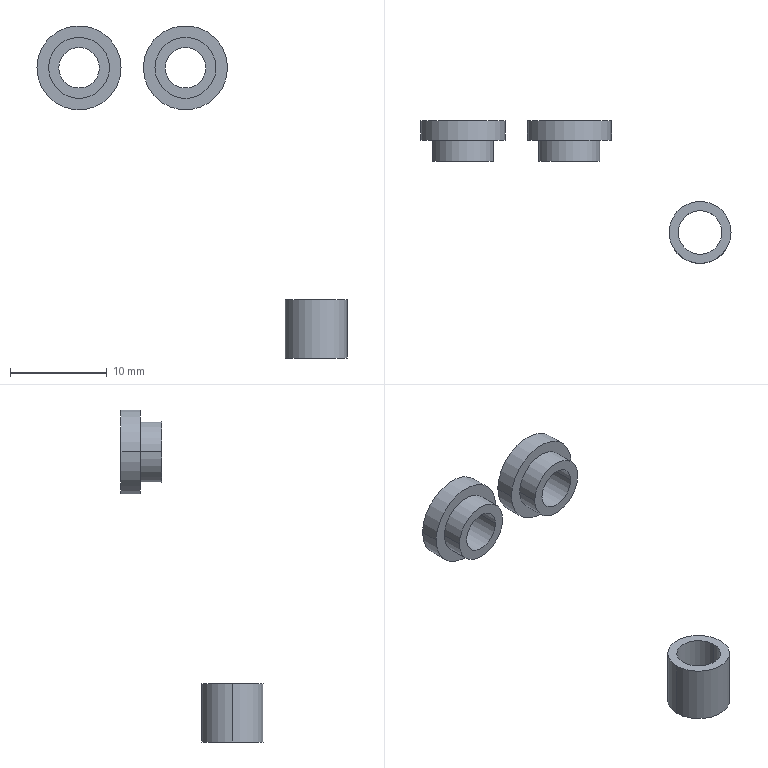Part | NX | features BREP 3 | 3 solids | 24 faces | box 32.05 x 14.7 x 34.343 mm | volume 356.162 mm3 | cylinder 16 | plane 8 | commonest cylinder face diameters 4.2 x4 6.3 x4 8.7 x4 4.5 x2 6.4 x2
STEP:
#1=CARTESIAN_POINT('',(49.941,-46.741,33.83));
#2=VERTEX_POINT('',#1);
#3=CARTESIAN_POINT('',(43.541,-46.741,33.83));
#4=VERTEX_POINT('',#3);
#5=CARTESIAN_POINT('',(46.741,-46.741,33.83));
#6=DIRECTION('',(0.,0.,1.));
#7=DIRECTION('',(1.,0.,0.));
#8=AXIS2_PLACEMENT_3D('',#5,#6,#7);
#9=CIRCLE('',#8,3.2);
#10=EDGE_CURVE('',#2,#4,#9,.T.);
#11=ORIENTED_EDGE('',*,*,#10,.T.);
#12=CARTESIAN_POINT('',(46.741,-46.741,33.83));
#13=DIRECTION('',(0.,0.,1.));
#14=DIRECTION('',(-1.,0.,0.));
#15=AXIS2_PLACEMENT_3D('',#12,#13,#14);
#16=CIRCLE('',#15,3.2);
#17=EDGE_CURVE('',#4,#2,#16,.T.);
#18=ORIENTED_EDGE('',*,*,#17,.T.);
#19=EDGE_LOOP('',(#11,#18));
#20=FACE_BOUND('',#19,.T.);
#21=CARTESIAN_POINT('',(48.991,-46.741,33.83));
#22=VERTEX_POINT('',#21);
#23=CARTESIAN_POINT('',(44.491,-46.741,33.83));
#24=VERTEX_POINT('',#23);
#25=CARTESIAN_POINT('',(46.741,-46.741,33.83));
#26=DIRECTION('',(0.,0.,-1.));
#27=DIRECTION('',(1.,0.,0.));
#28=AXIS2_PLACEMENT_3D('',#25,#26,#27);
#29=CIRCLE('',#28,2.25);
#30=EDGE_CURVE('',#22,#24,#29,.T.);
#31=ORIENTED_EDGE('',*,*,#30,.T.);
#32=CARTESIAN_POINT('',(46.741,-46.741,33.83));
#33=DIRECTION('',(0.,0.,-1.));
#34=DIRECTION('',(-1.,0.,0.));
#35=AXIS2_PLACEMENT_3D('',#32,#33,#34);
#36=CIRCLE('',#35,2.25);
#37=EDGE_CURVE('',#24,#22,#36,.T.);
#38=ORIENTED_EDGE('',*,*,#37,.T.);
#39=EDGE_LOOP('',(#31,#38));
#40=FACE_BOUND('',#39,.T.);
#41=CARTESIAN_POINT('',(0.,0.,33.83));
#42=DIRECTION('',(0.,0.,1.));
#43=DIRECTION('',(1.,0.,0.));
#44=AXIS2_PLACEMENT_3D('',#41,#42,#43);
#45=PLANE('',#44);
#46=ADVANCED_FACE('',(#20,#40),#45,.T.);
#47=CARTESIAN_POINT('',(49.941,-46.741,27.83));
#48=VERTEX_POINT('',#47);
#49=CARTESIAN_POINT('',(43.541,-46.741,27.83));
#50=VERTEX_POINT('',#49);
#51=CARTESIAN_POINT('',(46.741,-46.741,27.83));
#52=DIRECTION('',(0.,0.,-1.));
#53=DIRECTION('',(1.,0.,0.));
#54=AXIS2_PLACEMENT_3D('',#51,#52,#53);
#55=CIRCLE('',#54,3.2);
#56=EDGE_CURVE('',#48,#50,#55,.T.);
#57=ORIENTED_EDGE('',*,*,#56,.F.);
#58=CARTESIAN_POINT('',(49.941,-46.741,33.83));
#59=DIRECTION('',(0.,0.,-1.));
#60=VECTOR('',#59,1000.);
#61=LINE('',#58,#60);
#62=EDGE_CURVE('',#2,#48,#61,.T.);
#63=ORIENTED_EDGE('',*,*,#62,.F.);
#64=ORIENTED_EDGE('',*,*,#17,.F.);
#65=CARTESIAN_POINT('',(43.541,-46.741,33.83));
#66=DIRECTION('',(0.,0.,-1.));
#67=VECTOR('',#66,1000.);
#68=LINE('',#65,#67);
#69=EDGE_CURVE('',#4,#50,#68,.T.);
#70=ORIENTED_EDGE('',*,*,#69,.T.);
#71=EDGE_LOOP('',(#57,#63,#64,#70));
#72=FACE_BOUND('',#71,.T.);
#73=CARTESIAN_POINT('',(46.741,-46.741,33.83));
#74=DIRECTION('',(0.,0.,1.));
#75=DIRECTION('',(1.,0.,0.));
#76=AXIS2_PLACEMENT_3D('',#73,#74,#75);
#77=CYLINDRICAL_SURFACE('',#76,3.2);
#78=ADVANCED_FACE('',(#72),#77,.T.);
#79=CARTESIAN_POINT('',(46.741,-46.741,27.83));
#80=DIRECTION('',(0.,0.,-1.));
#81=DIRECTION('',(-1.,0.,0.));
#82=AXIS2_PLACEMENT_3D('',#79,#80,#81);
#83=CIRCLE('',#82,3.2);
#84=EDGE_CURVE('',#50,#48,#83,.T.);
#85=ORIENTED_EDGE('',*,*,#84,.F.);
#86=ORIENTED_EDGE('',*,*,#69,.F.);
#87=ORIENTED_EDGE('',*,*,#10,.F.);
#88=ORIENTED_EDGE('',*,*,#62,.T.);
#89=EDGE_LOOP('',(#85,#86,#87,#88));
#90=FACE_BOUND('',#89,.T.);
#91=CARTESIAN_POINT('',(46.741,-46.741,33.83));
#92=DIRECTION('',(0.,0.,1.));
#93=DIRECTION('',(1.,0.,0.));
#94=AXIS2_PLACEMENT_3D('',#91,#92,#93);
#95=CYLINDRICAL_SURFACE('',#94,3.2);
#96=ADVANCED_FACE('',(#90),#95,.T.);
#97=ORIENTED_EDGE('',*,*,#84,.T.);
#98=ORIENTED_EDGE('',*,*,#56,.T.);
#99=EDGE_LOOP('',(#97,#98));
#100=FACE_BOUND('',#99,.T.);
#101=CARTESIAN_POINT('',(44.491,-46.741,27.83));
#102=VERTEX_POINT('',#101);
#103=CARTESIAN_POINT('',(48.991,-46.741,27.83));
#104=VERTEX_POINT('',#103);
#105=CARTESIAN_POINT('',(46.741,-46.741,27.83));
#106=DIRECTION('',(0.,0.,1.));
#107=DIRECTION('',(-1.,0.,0.));
#108=AXIS2_PLACEMENT_3D('',#105,#106,#107);
#109=CIRCLE('',#108,2.25);
#110=EDGE_CURVE('',#102,#104,#109,.T.);
#111=ORIENTED_EDGE('',*,*,#110,.T.);
#112=CARTESIAN_POINT('',(46.741,-46.741,27.83));
#113=DIRECTION('',(0.,0.,1.));
#114=DIRECTION('',(1.,0.,0.));
#115=AXIS2_PLACEMENT_3D('',#112,#113,#114);
#116=CIRCLE('',#115,2.25);
#117=EDGE_CURVE('',#104,#102,#116,.T.);
#118=ORIENTED_EDGE('',*,*,#117,.T.);
#119=EDGE_LOOP('',(#111,#118));
#120=FACE_BOUND('',#119,.T.);
#121=CARTESIAN_POINT('',(0.,0.,27.83));
#122=DIRECTION('',(0.,0.,1.));
#123=DIRECTION('',(1.,0.,0.));
#124=AXIS2_PLACEMENT_3D('',#121,#122,#123);
#125=PLANE('',#124);
#126=ADVANCED_FACE('',(#100,#120),#125,.F.);
#127=ORIENTED_EDGE('',*,*,#117,.F.);
#128=CARTESIAN_POINT('',(48.991,-46.741,33.83));
#129=DIRECTION('',(0.,0.,-1.));
#130=VECTOR('',#129,1000.);
#131=LINE('',#128,#130);
#132=EDGE_CURVE('',#22,#104,#131,.T.);
#133=ORIENTED_EDGE('',*,*,#132,.F.);
#134=ORIENTED_EDGE('',*,*,#37,.F.);
#135=CARTESIAN_POINT('',(44.491,-46.741,33.83));
#136=DIRECTION('',(0.,0.,-1.));
#137=VECTOR('',#136,1000.);
#138=LINE('',#135,#137);
#139=EDGE_CURVE('',#24,#102,#138,.T.);
#140=ORIENTED_EDGE('',*,*,#139,.T.);
#141=EDGE_LOOP('',(#127,#133,#134,#140));
#142=FACE_BOUND('',#141,.T.);
#143=CARTESIAN_POINT('',(46.741,-46.741,33.83));
#144=DIRECTION('',(0.,0.,1.));
#145=DIRECTION('',(1.,0.,0.));
#146=AXIS2_PLACEMENT_3D('',#143,#144,#145);
#147=CYLINDRICAL_SURFACE('',#146,2.25);
#148=ADVANCED_FACE('',(#142),#147,.F.);
#149=ORIENTED_EDGE('',*,*,#110,.F.);
#150=ORIENTED_EDGE('',*,*,#139,.F.);
#151=ORIENTED_EDGE('',*,*,#30,.F.);
#152=ORIENTED_EDGE('',*,*,#132,.T.);
#153=EDGE_LOOP('',(#149,#150,#151,#152));
#154=FACE_BOUND('',#153,.T.);
#155=CARTESIAN_POINT('',(46.741,-46.741,33.83));
#156=DIRECTION('',(0.,0.,1.));
#157=DIRECTION('',(1.,0.,0.));
#158=AXIS2_PLACEMENT_3D('',#155,#156,#157);
#159=CYLINDRICAL_SURFACE('',#158,2.25);
#160=ADVANCED_FACE('',(#154),#159,.F.);
#161=CLOSED_SHELL('',(#46,#78,#96,#126,#148,#160));
#162=MANIFOLD_SOLID_BREP('',#161);
#163=CARTESIAN_POINT('',(26.591,-37.241,57.823));
#164=VERTEX_POINT('',#163);
#165=CARTESIAN_POINT('',(17.891,-37.241,57.823));
#166=VERTEX_POINT('',#165);
#167=CARTESIAN_POINT('',(22.241,-37.241,57.823));
#168=DIRECTION('',(0.,1.,0.));
#169=DIRECTION('',(1.,0.,0.));
#170=AXIS2_PLACEMENT_3D('',#167,#168,#169);
#171=CIRCLE('',#170,4.35);
#172=EDGE_CURVE('',#164,#166,#171,.T.);
#173=ORIENTED_EDGE('',*,*,#172,.F.);
#174=CARTESIAN_POINT('',(22.241,-37.241,57.823));
#175=DIRECTION('',(0.,1.,0.));
#176=DIRECTION('',(-1.,0.,0.));
#177=AXIS2_PLACEMENT_3D('',#174,#175,#176);
#178=CIRCLE('',#177,4.35);
#179=EDGE_CURVE('',#166,#164,#178,.T.);
#180=ORIENTED_EDGE('',*,*,#179,.F.);
#181=EDGE_LOOP('',(#173,#180));
#182=FACE_BOUND('',#181,.T.);
#183=CARTESIAN_POINT('',(19.091,-37.241,57.823));
#184=VERTEX_POINT('',#183);
#185=CARTESIAN_POINT('',(25.391,-37.241,57.823));
#186=VERTEX_POINT('',#185);
#187=CARTESIAN_POINT('',(22.241,-37.241,57.823));
#188=DIRECTION('',(0.,-1.,0.));
#189=DIRECTION('',(-1.,0.,0.));
#190=AXIS2_PLACEMENT_3D('',#187,#188,#189);
#191=CIRCLE('',#190,3.15);
#192=EDGE_CURVE('',#184,#186,#191,.T.);
#193=ORIENTED_EDGE('',*,*,#192,.F.);
#194=CARTESIAN_POINT('',(22.241,-37.241,57.823));
#195=DIRECTION('',(0.,-1.,0.));
#196=DIRECTION('',(1.,0.,0.));
#197=AXIS2_PLACEMENT_3D('',#194,#195,#196);
#198=CIRCLE('',#197,3.15);
#199=EDGE_CURVE('',#186,#184,#198,.T.);
#200=ORIENTED_EDGE('',*,*,#199,.F.);
#201=EDGE_LOOP('',(#193,#200));
#202=FACE_BOUND('',#201,.T.);
#203=CARTESIAN_POINT('',(0.,-37.241,0.));
#204=DIRECTION('',(0.,1.,0.));
#205=DIRECTION('',(1.,0.,0.));
#206=AXIS2_PLACEMENT_3D('',#203,#204,#205);
#207=PLANE('',#206);
#208=ADVANCED_FACE('',(#182,#202),#207,.F.);
#209=CARTESIAN_POINT('',(26.591,-35.241,57.823));
#210=VERTEX_POINT('',#209);
#211=CARTESIAN_POINT('',(26.591,-37.241,57.823));
#212=DIRECTION('',(0.,-1.,0.));
#213=VECTOR('',#212,1000.);
#214=LINE('',#211,#213);
#215=EDGE_CURVE('',#210,#164,#214,.T.);
#216=ORIENTED_EDGE('',*,*,#215,.F.);
#217=CARTESIAN_POINT('',(17.891,-35.241,57.823));
#218=VERTEX_POINT('',#217);
#219=CARTESIAN_POINT('',(22.241,-35.241,57.823));
#220=DIRECTION('',(0.,1.,0.));
#221=DIRECTION('',(-1.,0.,0.));
#222=AXIS2_PLACEMENT_3D('',#219,#220,#221);
#223=CIRCLE('',#222,4.35);
#224=EDGE_CURVE('',#218,#210,#223,.T.);
#225=ORIENTED_EDGE('',*,*,#224,.F.);
#226=CARTESIAN_POINT('',(17.891,-37.241,57.823));
#227=DIRECTION('',(0.,-1.,0.));
#228=VECTOR('',#227,1000.);
#229=LINE('',#226,#228);
#230=EDGE_CURVE('',#218,#166,#229,.T.);
#231=ORIENTED_EDGE('',*,*,#230,.T.);
#232=ORIENTED_EDGE('',*,*,#179,.T.);
#233=EDGE_LOOP('',(#216,#225,#231,#232));
#234=FACE_BOUND('',#233,.T.);
#235=CARTESIAN_POINT('',(22.241,-37.241,57.823));
#236=DIRECTION('',(0.,1.,0.));
#237=DIRECTION('',(1.,0.,0.));
#238=AXIS2_PLACEMENT_3D('',#235,#236,#237);
#239=CYLINDRICAL_SURFACE('',#238,4.35);
#240=ADVANCED_FACE('',(#234),#239,.T.);
#241=ORIENTED_EDGE('',*,*,#230,.F.);
#242=CARTESIAN_POINT('',(22.241,-35.241,57.823));
#243=DIRECTION('',(0.,1.,0.));
#244=DIRECTION('',(1.,0.,0.));
#245=AXIS2_PLACEMENT_3D('',#242,#243,#244);
#246=CIRCLE('',#245,4.35);
#247=EDGE_CURVE('',#210,#218,#246,.T.);
#248=ORIENTED_EDGE('',*,*,#247,.F.);
#249=ORIENTED_EDGE('',*,*,#215,.T.);
#250=ORIENTED_EDGE('',*,*,#172,.T.);
#251=EDGE_LOOP('',(#241,#248,#249,#250));
#252=FACE_BOUND('',#251,.T.);
#253=CARTESIAN_POINT('',(22.241,-37.241,57.823));
#254=DIRECTION('',(0.,1.,0.));
#255=DIRECTION('',(1.,0.,0.));
#256=AXIS2_PLACEMENT_3D('',#253,#254,#255);
#257=CYLINDRICAL_SURFACE('',#256,4.35);
#258=ADVANCED_FACE('',(#252),#257,.T.);
#259=ORIENTED_EDGE('',*,*,#247,.T.);
#260=ORIENTED_EDGE('',*,*,#224,.T.);
#261=EDGE_LOOP('',(#259,#260));
#262=FACE_BOUND('',#261,.T.);
#263=CARTESIAN_POINT('',(24.341,-35.241,57.823));
#264=VERTEX_POINT('',#263);
#265=CARTESIAN_POINT('',(20.141,-35.241,57.823));
#266=VERTEX_POINT('',#265);
#267=CARTESIAN_POINT('',(22.241,-35.241,57.823));
#268=DIRECTION('',(0.,-1.,0.));
#269=DIRECTION('',(1.,0.,0.));
#270=AXIS2_PLACEMENT_3D('',#267,#268,#269);
#271=CIRCLE('',#270,2.1);
#272=EDGE_CURVE('',#264,#266,#271,.T.);
#273=ORIENTED_EDGE('',*,*,#272,.T.);
#274=CARTESIAN_POINT('',(22.241,-35.241,57.823));
#275=DIRECTION('',(0.,-1.,0.));
#276=DIRECTION('',(-1.,0.,0.));
#277=AXIS2_PLACEMENT_3D('',#274,#275,#276);
#278=CIRCLE('',#277,2.1);
#279=EDGE_CURVE('',#266,#264,#278,.T.);
#280=ORIENTED_EDGE('',*,*,#279,.T.);
#281=EDGE_LOOP('',(#273,#280));
#282=FACE_BOUND('',#281,.T.);
#283=CARTESIAN_POINT('',(0.,-35.241,0.));
#284=DIRECTION('',(0.,1.,0.));
#285=DIRECTION('',(1.,0.,0.));
#286=AXIS2_PLACEMENT_3D('',#283,#284,#285);
#287=PLANE('',#286);
#288=ADVANCED_FACE('',(#262,#282),#287,.T.);
#289=ORIENTED_EDGE('',*,*,#279,.F.);
#290=CARTESIAN_POINT('',(20.141,-39.441,57.823));
#291=VERTEX_POINT('',#290);
#292=CARTESIAN_POINT('',(20.141,-35.241,57.823));
#293=DIRECTION('',(0.,-1.,0.));
#294=VECTOR('',#293,1000.);
#295=LINE('',#292,#294);
#296=EDGE_CURVE('',#266,#291,#295,.T.);
#297=ORIENTED_EDGE('',*,*,#296,.T.);
#298=CARTESIAN_POINT('',(24.341,-39.441,57.823));
#299=VERTEX_POINT('',#298);
#300=CARTESIAN_POINT('',(22.241,-39.441,57.823));
#301=DIRECTION('',(0.,1.,0.));
#302=DIRECTION('',(1.,0.,0.));
#303=AXIS2_PLACEMENT_3D('',#300,#301,#302);
#304=CIRCLE('',#303,2.1);
#305=EDGE_CURVE('',#299,#291,#304,.T.);
#306=ORIENTED_EDGE('',*,*,#305,.F.);
#307=CARTESIAN_POINT('',(24.341,-39.441,57.823));
#308=DIRECTION('',(0.,1.,0.));
#309=VECTOR('',#308,1000.);
#310=LINE('',#307,#309);
#311=EDGE_CURVE('',#299,#264,#310,.T.);
#312=ORIENTED_EDGE('',*,*,#311,.T.);
#313=EDGE_LOOP('',(#289,#297,#306,#312));
#314=FACE_BOUND('',#313,.T.);
#315=CARTESIAN_POINT('',(22.241,-37.241,57.823));
#316=DIRECTION('',(0.,1.,0.));
#317=DIRECTION('',(1.,0.,0.));
#318=AXIS2_PLACEMENT_3D('',#315,#316,#317);
#319=CYLINDRICAL_SURFACE('',#318,2.1);
#320=ADVANCED_FACE('',(#314),#319,.F.);
#321=ORIENTED_EDGE('',*,*,#272,.F.);
#322=ORIENTED_EDGE('',*,*,#311,.F.);
#323=CARTESIAN_POINT('',(22.241,-39.441,57.823));
#324=DIRECTION('',(0.,1.,0.));
#325=DIRECTION('',(-1.,0.,0.));
#326=AXIS2_PLACEMENT_3D('',#323,#324,#325);
#327=CIRCLE('',#326,2.1);
#328=EDGE_CURVE('',#291,#299,#327,.T.);
#329=ORIENTED_EDGE('',*,*,#328,.F.);
#330=ORIENTED_EDGE('',*,*,#296,.F.);
#331=EDGE_LOOP('',(#321,#322,#329,#330));
#332=FACE_BOUND('',#331,.T.);
#333=CARTESIAN_POINT('',(22.241,-37.241,57.823));
#334=DIRECTION('',(0.,1.,0.));
#335=DIRECTION('',(1.,0.,0.));
#336=AXIS2_PLACEMENT_3D('',#333,#334,#335);
#337=CYLINDRICAL_SURFACE('',#336,2.1);
#338=ADVANCED_FACE('',(#332),#337,.F.);
#339=CARTESIAN_POINT('',(19.091,-39.441,57.823));
#340=VERTEX_POINT('',#339);
#341=CARTESIAN_POINT('',(25.391,-39.441,57.823));
#342=VERTEX_POINT('',#341);
#343=CARTESIAN_POINT('',(22.241,-39.441,57.823));
#344=DIRECTION('',(0.,-1.,0.));
#345=DIRECTION('',(-1.,0.,0.));
#346=AXIS2_PLACEMENT_3D('',#343,#344,#345);
#347=CIRCLE('',#346,3.15);
#348=EDGE_CURVE('',#340,#342,#347,.T.);
#349=ORIENTED_EDGE('',*,*,#348,.T.);
#350=CARTESIAN_POINT('',(22.241,-39.441,57.823));
#351=DIRECTION('',(0.,-1.,0.));
#352=DIRECTION('',(1.,0.,0.));
#353=AXIS2_PLACEMENT_3D('',#350,#351,#352);
#354=CIRCLE('',#353,3.15);
#355=EDGE_CURVE('',#342,#340,#354,.T.);
#356=ORIENTED_EDGE('',*,*,#355,.T.);
#357=EDGE_LOOP('',(#349,#356));
#358=FACE_BOUND('',#357,.T.);
#359=ORIENTED_EDGE('',*,*,#328,.T.);
#360=ORIENTED_EDGE('',*,*,#305,.T.);
#361=EDGE_LOOP('',(#359,#360));
#362=FACE_BOUND('',#361,.T.);
#363=CARTESIAN_POINT('',(0.,-39.441,0.));
#364=DIRECTION('',(0.,-1.,0.));
#365=DIRECTION('',(-1.,0.,0.));
#366=AXIS2_PLACEMENT_3D('',#363,#364,#365);
#367=PLANE('',#366);
#368=ADVANCED_FACE('',(#358,#362),#367,.T.);
#369=CARTESIAN_POINT('',(19.091,-37.241,57.823));
#370=DIRECTION('',(0.,-1.,0.));
#371=VECTOR('',#370,1000.);
#372=LINE('',#369,#371);
#373=EDGE_CURVE('',#184,#340,#372,.T.);
#374=ORIENTED_EDGE('',*,*,#373,.T.);
#375=ORIENTED_EDGE('',*,*,#355,.F.);
#376=CARTESIAN_POINT('',(25.391,-37.241,57.823));
#377=DIRECTION('',(0.,-1.,0.));
#378=VECTOR('',#377,1000.);
#379=LINE('',#376,#378);
#380=EDGE_CURVE('',#186,#342,#379,.T.);
#381=ORIENTED_EDGE('',*,*,#380,.F.);
#382=ORIENTED_EDGE('',*,*,#199,.T.);
#383=EDGE_LOOP('',(#374,#375,#381,#382));
#384=FACE_BOUND('',#383,.T.);
#385=CARTESIAN_POINT('',(22.241,-37.241,57.823));
#386=DIRECTION('',(0.,-1.,0.));
#387=DIRECTION('',(-1.,0.,0.));
#388=AXIS2_PLACEMENT_3D('',#385,#386,#387);
#389=CYLINDRICAL_SURFACE('',#388,3.15);
#390=ADVANCED_FACE('',(#384),#389,.T.);
#391=ORIENTED_EDGE('',*,*,#380,.T.);
#392=ORIENTED_EDGE('',*,*,#348,.F.);
#393=ORIENTED_EDGE('',*,*,#373,.F.);
#394=ORIENTED_EDGE('',*,*,#192,.T.);
#395=EDGE_LOOP('',(#391,#392,#393,#394));
#396=FACE_BOUND('',#395,.T.);
#397=CARTESIAN_POINT('',(22.241,-37.241,57.823));
#398=DIRECTION('',(0.,-1.,0.));
#399=DIRECTION('',(-1.,0.,0.));
#400=AXIS2_PLACEMENT_3D('',#397,#398,#399);
#401=CYLINDRICAL_SURFACE('',#400,3.15);
#402=ADVANCED_FACE('',(#396),#401,.T.);
#403=CLOSED_SHELL('',(#208,#240,#258,#288,#320,#338,#368,#390,#402));
#404=MANIFOLD_SOLID_BREP('',#403);
#405=CARTESIAN_POINT('',(37.591,-37.241,57.823));
#406=VERTEX_POINT('',#405);
#407=CARTESIAN_POINT('',(28.891,-37.241,57.823));
#408=VERTEX_POINT('',#407);
#409=CARTESIAN_POINT('',(33.241,-37.241,57.823));
#410=DIRECTION('',(0.,1.,0.));
#411=DIRECTION('',(1.,0.,0.));
#412=AXIS2_PLACEMENT_3D('',#409,#410,#411);
#413=CIRCLE('',#412,4.35);
#414=EDGE_CURVE('',#406,#408,#413,.T.);
#415=ORIENTED_EDGE('',*,*,#414,.F.);
#416=CARTESIAN_POINT('',(33.241,-37.241,57.823));
#417=DIRECTION('',(0.,1.,0.));
#418=DIRECTION('',(-1.,0.,0.));
#419=AXIS2_PLACEMENT_3D('',#416,#417,#418);
#420=CIRCLE('',#419,4.35);
#421=EDGE_CURVE('',#408,#406,#420,.T.);
#422=ORIENTED_EDGE('',*,*,#421,.F.);
#423=EDGE_LOOP('',(#415,#422));
#424=FACE_BOUND('',#423,.T.);
#425=CARTESIAN_POINT('',(30.091,-37.241,57.823));
#426=VERTEX_POINT('',#425);
#427=CARTESIAN_POINT('',(36.391,-37.241,57.823));
#428=VERTEX_POINT('',#427);
#429=CARTESIAN_POINT('',(33.241,-37.241,57.823));
#430=DIRECTION('',(0.,-1.,0.));
#431=DIRECTION('',(-1.,0.,0.));
#432=AXIS2_PLACEMENT_3D('',#429,#430,#431);
#433=CIRCLE('',#432,3.15);
#434=EDGE_CURVE('',#426,#428,#433,.T.);
#435=ORIENTED_EDGE('',*,*,#434,.F.);
#436=CARTESIAN_POINT('',(33.241,-37.241,57.823));
#437=DIRECTION('',(0.,-1.,0.));
#438=DIRECTION('',(1.,0.,0.));
#439=AXIS2_PLACEMENT_3D('',#436,#437,#438);
#440=CIRCLE('',#439,3.15);
#441=EDGE_CURVE('',#428,#426,#440,.T.);
#442=ORIENTED_EDGE('',*,*,#441,.F.);
#443=EDGE_LOOP('',(#435,#442));
#444=FACE_BOUND('',#443,.T.);
#445=CARTESIAN_POINT('',(0.,-37.241,0.));
#446=DIRECTION('',(0.,1.,0.));
#447=DIRECTION('',(1.,0.,0.));
#448=AXIS2_PLACEMENT_3D('',#445,#446,#447);
#449=PLANE('',#448);
#450=ADVANCED_FACE('',(#424,#444),#449,.F.);
#451=CARTESIAN_POINT('',(37.591,-35.241,57.823));
#452=VERTEX_POINT('',#451);
#453=CARTESIAN_POINT('',(37.591,-37.241,57.823));
#454=DIRECTION('',(0.,-1.,0.));
#455=VECTOR('',#454,1000.);
#456=LINE('',#453,#455);
#457=EDGE_CURVE('',#452,#406,#456,.T.);
#458=ORIENTED_EDGE('',*,*,#457,.F.);
#459=CARTESIAN_POINT('',(28.891,-35.241,57.823));
#460=VERTEX_POINT('',#459);
#461=CARTESIAN_POINT('',(33.241,-35.241,57.823));
#462=DIRECTION('',(0.,1.,0.));
#463=DIRECTION('',(-1.,0.,0.));
#464=AXIS2_PLACEMENT_3D('',#461,#462,#463);
#465=CIRCLE('',#464,4.35);
#466=EDGE_CURVE('',#460,#452,#465,.T.);
#467=ORIENTED_EDGE('',*,*,#466,.F.);
#468=CARTESIAN_POINT('',(28.891,-37.241,57.823));
#469=DIRECTION('',(0.,-1.,0.));
#470=VECTOR('',#469,1000.);
#471=LINE('',#468,#470);
#472=EDGE_CURVE('',#460,#408,#471,.T.);
#473=ORIENTED_EDGE('',*,*,#472,.T.);
#474=ORIENTED_EDGE('',*,*,#421,.T.);
#475=EDGE_LOOP('',(#458,#467,#473,#474));
#476=FACE_BOUND('',#475,.T.);
#477=CARTESIAN_POINT('',(33.241,-37.241,57.823));
#478=DIRECTION('',(0.,1.,0.));
#479=DIRECTION('',(1.,0.,0.));
#480=AXIS2_PLACEMENT_3D('',#477,#478,#479);
#481=CYLINDRICAL_SURFACE('',#480,4.35);
#482=ADVANCED_FACE('',(#476),#481,.T.);
#483=ORIENTED_EDGE('',*,*,#472,.F.);
#484=CARTESIAN_POINT('',(33.241,-35.241,57.823));
#485=DIRECTION('',(0.,1.,0.));
#486=DIRECTION('',(1.,0.,0.));
#487=AXIS2_PLACEMENT_3D('',#484,#485,#486);
#488=CIRCLE('',#487,4.35);
#489=EDGE_CURVE('',#452,#460,#488,.T.);
#490=ORIENTED_EDGE('',*,*,#489,.F.);
#491=ORIENTED_EDGE('',*,*,#457,.T.);
#492=ORIENTED_EDGE('',*,*,#414,.T.);
#493=EDGE_LOOP('',(#483,#490,#491,#492));
#494=FACE_BOUND('',#493,.T.);
#495=CARTESIAN_POINT('',(33.241,-37.241,57.823));
#496=DIRECTION('',(0.,1.,0.));
#497=DIRECTION('',(1.,0.,0.));
#498=AXIS2_PLACEMENT_3D('',#495,#496,#497);
#499=CYLINDRICAL_SURFACE('',#498,4.35);
#500=ADVANCED_FACE('',(#494),#499,.T.);
#501=ORIENTED_EDGE('',*,*,#489,.T.);
#502=ORIENTED_EDGE('',*,*,#466,.T.);
#503=EDGE_LOOP('',(#501,#502));
#504=FACE_BOUND('',#503,.T.);
#505=CARTESIAN_POINT('',(35.341,-35.241,57.823));
#506=VERTEX_POINT('',#505);
#507=CARTESIAN_POINT('',(31.141,-35.241,57.823));
#508=VERTEX_POINT('',#507);
#509=CARTESIAN_POINT('',(33.241,-35.241,57.823));
#510=DIRECTION('',(0.,-1.,0.));
#511=DIRECTION('',(1.,0.,0.));
#512=AXIS2_PLACEMENT_3D('',#509,#510,#511);
#513=CIRCLE('',#512,2.1);
#514=EDGE_CURVE('',#506,#508,#513,.T.);
#515=ORIENTED_EDGE('',*,*,#514,.T.);
#516=CARTESIAN_POINT('',(33.241,-35.241,57.823));
#517=DIRECTION('',(0.,-1.,0.));
#518=DIRECTION('',(-1.,0.,0.));
#519=AXIS2_PLACEMENT_3D('',#516,#517,#518);
#520=CIRCLE('',#519,2.1);
#521=EDGE_CURVE('',#508,#506,#520,.T.);
#522=ORIENTED_EDGE('',*,*,#521,.T.);
#523=EDGE_LOOP('',(#515,#522));
#524=FACE_BOUND('',#523,.T.);
#525=CARTESIAN_POINT('',(0.,-35.241,0.));
#526=DIRECTION('',(0.,1.,0.));
#527=DIRECTION('',(1.,0.,0.));
#528=AXIS2_PLACEMENT_3D('',#525,#526,#527);
#529=PLANE('',#528);
#530=ADVANCED_FACE('',(#504,#524),#529,.T.);
#531=ORIENTED_EDGE('',*,*,#521,.F.);
#532=CARTESIAN_POINT('',(31.141,-39.441,57.823));
#533=VERTEX_POINT('',#532);
#534=CARTESIAN_POINT('',(31.141,-35.241,57.823));
#535=DIRECTION('',(0.,-1.,0.));
#536=VECTOR('',#535,1000.);
#537=LINE('',#534,#536);
#538=EDGE_CURVE('',#508,#533,#537,.T.);
#539=ORIENTED_EDGE('',*,*,#538,.T.);
#540=CARTESIAN_POINT('',(35.341,-39.441,57.823));
#541=VERTEX_POINT('',#540);
#542=CARTESIAN_POINT('',(33.241,-39.441,57.823));
#543=DIRECTION('',(0.,1.,0.));
#544=DIRECTION('',(1.,0.,0.));
#545=AXIS2_PLACEMENT_3D('',#542,#543,#544);
#546=CIRCLE('',#545,2.1);
#547=EDGE_CURVE('',#541,#533,#546,.T.);
#548=ORIENTED_EDGE('',*,*,#547,.F.);
#549=CARTESIAN_POINT('',(35.341,-39.441,57.823));
#550=DIRECTION('',(0.,1.,0.));
#551=VECTOR('',#550,1000.);
#552=LINE('',#549,#551);
#553=EDGE_CURVE('',#541,#506,#552,.T.);
#554=ORIENTED_EDGE('',*,*,#553,.T.);
#555=EDGE_LOOP('',(#531,#539,#548,#554));
#556=FACE_BOUND('',#555,.T.);
#557=CARTESIAN_POINT('',(33.241,-37.241,57.823));
#558=DIRECTION('',(0.,1.,0.));
#559=DIRECTION('',(1.,0.,0.));
#560=AXIS2_PLACEMENT_3D('',#557,#558,#559);
#561=CYLINDRICAL_SURFACE('',#560,2.1);
#562=ADVANCED_FACE('',(#556),#561,.F.);
#563=ORIENTED_EDGE('',*,*,#514,.F.);
#564=ORIENTED_EDGE('',*,*,#553,.F.);
#565=CARTESIAN_POINT('',(33.241,-39.441,57.823));
#566=DIRECTION('',(0.,1.,0.));
#567=DIRECTION('',(-1.,0.,0.));
#568=AXIS2_PLACEMENT_3D('',#565,#566,#567);
#569=CIRCLE('',#568,2.1);
#570=EDGE_CURVE('',#533,#541,#569,.T.);
#571=ORIENTED_EDGE('',*,*,#570,.F.);
#572=ORIENTED_EDGE('',*,*,#538,.F.);
#573=EDGE_LOOP('',(#563,#564,#571,#572));
#574=FACE_BOUND('',#573,.T.);
#575=CARTESIAN_POINT('',(33.241,-37.241,57.823));
#576=DIRECTION('',(0.,1.,0.));
#577=DIRECTION('',(1.,0.,0.));
#578=AXIS2_PLACEMENT_3D('',#575,#576,#577);
#579=CYLINDRICAL_SURFACE('',#578,2.1);
#580=ADVANCED_FACE('',(#574),#579,.F.);
#581=CARTESIAN_POINT('',(30.091,-39.441,57.823));
#582=VERTEX_POINT('',#581);
#583=CARTESIAN_POINT('',(36.391,-39.441,57.823));
#584=VERTEX_POINT('',#583);
#585=CARTESIAN_POINT('',(33.241,-39.441,57.823));
#586=DIRECTION('',(0.,-1.,0.));
#587=DIRECTION('',(-1.,0.,0.));
#588=AXIS2_PLACEMENT_3D('',#585,#586,#587);
#589=CIRCLE('',#588,3.15);
#590=EDGE_CURVE('',#582,#584,#589,.T.);
#591=ORIENTED_EDGE('',*,*,#590,.T.);
#592=CARTESIAN_POINT('',(33.241,-39.441,57.823));
#593=DIRECTION('',(0.,-1.,0.));
#594=DIRECTION('',(1.,0.,0.));
#595=AXIS2_PLACEMENT_3D('',#592,#593,#594);
#596=CIRCLE('',#595,3.15);
#597=EDGE_CURVE('',#584,#582,#596,.T.);
#598=ORIENTED_EDGE('',*,*,#597,.T.);
#599=EDGE_LOOP('',(#591,#598));
#600=FACE_BOUND('',#599,.T.);
#601=ORIENTED_EDGE('',*,*,#570,.T.);
#602=ORIENTED_EDGE('',*,*,#547,.T.);
#603=EDGE_LOOP('',(#601,#602));
#604=FACE_BOUND('',#603,.T.);
#605=CARTESIAN_POINT('',(0.,-39.441,0.));
#606=DIRECTION('',(0.,-1.,0.));
#607=DIRECTION('',(-1.,0.,0.));
#608=AXIS2_PLACEMENT_3D('',#605,#606,#607);
#609=PLANE('',#608);
#610=ADVANCED_FACE('',(#600,#604),#609,.T.);
#611=CARTESIAN_POINT('',(30.091,-37.241,57.823));
#612=DIRECTION('',(0.,-1.,0.));
#613=VECTOR('',#612,1000.);
#614=LINE('',#611,#613);
#615=EDGE_CURVE('',#426,#582,#614,.T.);
#616=ORIENTED_EDGE('',*,*,#615,.T.);
#617=ORIENTED_EDGE('',*,*,#597,.F.);
#618=CARTESIAN_POINT('',(36.391,-37.241,57.823));
#619=DIRECTION('',(0.,-1.,0.));
#620=VECTOR('',#619,1000.);
#621=LINE('',#618,#620);
#622=EDGE_CURVE('',#428,#584,#621,.T.);
#623=ORIENTED_EDGE('',*,*,#622,.F.);
#624=ORIENTED_EDGE('',*,*,#441,.T.);
#625=EDGE_LOOP('',(#616,#617,#623,#624));
#626=FACE_BOUND('',#625,.T.);
#627=CARTESIAN_POINT('',(33.241,-37.241,57.823));
#628=DIRECTION('',(0.,-1.,0.));
#629=DIRECTION('',(-1.,0.,0.));
#630=AXIS2_PLACEMENT_3D('',#627,#628,#629);
#631=CYLINDRICAL_SURFACE('',#630,3.15);
#632=ADVANCED_FACE('',(#626),#631,.T.);
#633=ORIENTED_EDGE('',*,*,#622,.T.);
#634=ORIENTED_EDGE('',*,*,#590,.F.);
#635=ORIENTED_EDGE('',*,*,#615,.F.);
#636=ORIENTED_EDGE('',*,*,#434,.T.);
#637=EDGE_LOOP('',(#633,#634,#635,#636));
#638=FACE_BOUND('',#637,.T.);
#639=CARTESIAN_POINT('',(33.241,-37.241,57.823));
#640=DIRECTION('',(0.,-1.,0.));
#641=DIRECTION('',(-1.,0.,0.));
#642=AXIS2_PLACEMENT_3D('',#639,#640,#641);
#643=CYLINDRICAL_SURFACE('',#642,3.15);
#644=ADVANCED_FACE('',(#638),#643,.T.);
#645=CLOSED_SHELL('',(#450,#482,#500,#530,#562,#580,#610,#632,#644));
#646=MANIFOLD_SOLID_BREP('',#645);
#647=(LENGTH_UNIT()NAMED_UNIT(*)SI_UNIT(.MILLI.,.METRE.));
#648=UNCERTAINTY_MEASURE_WITH_UNIT(LENGTH_MEASURE(0.00001),#647,'','');
#649=(NAMED_UNIT(*)PLANE_ANGLE_UNIT()SI_UNIT($,.RADIAN.));
#650=(NAMED_UNIT(*)SI_UNIT($,.STERADIAN.)SOLID_ANGLE_UNIT());
#651=(GEOMETRIC_REPRESENTATION_CONTEXT(3)GLOBAL_UNCERTAINTY_ASSIGNED_CONTEXT((#648))GLOBAL_UNIT_ASSIGNED_CONTEXT((#647,#649,#650))REPRESENTATION_CONTEXT('',''));
#652=ADVANCED_BREP_SHAPE_REPRESENTATION('',(#162,#404,#646),#651);